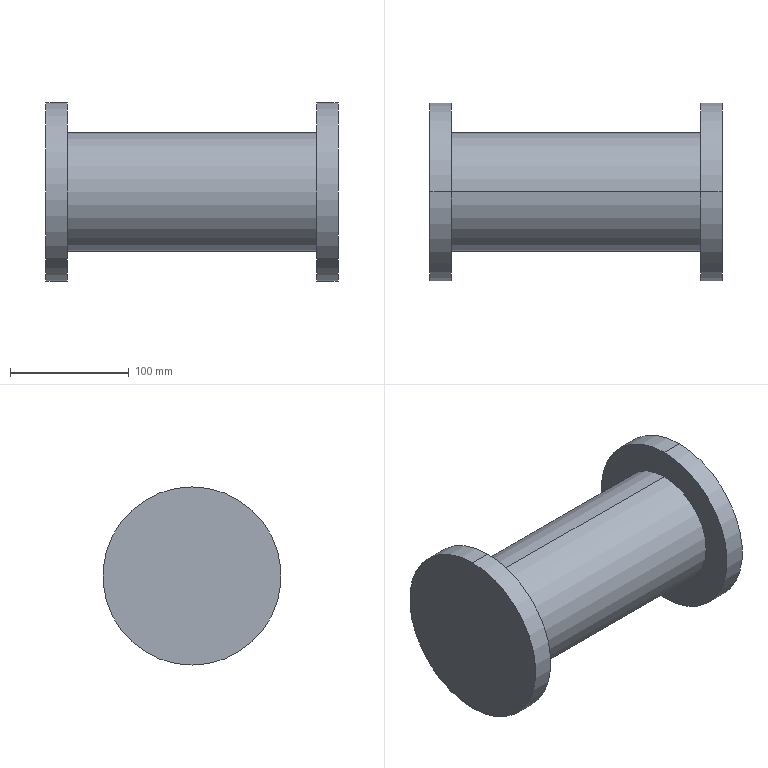Part | SolidWorks | features ICE 2, Extrusion 1 | 1 solid | 10 faces | box 246 x 150 x 150 mm | volume 2285509 mm3 | cylinder 6 | plane 4 | commonest cylinder face diameters 150 x4 100 x2
STEP:
#1=CARTESIAN_POINT('',(-228.,0.,-75.));
#2=VERTEX_POINT('',#1);
#3=CARTESIAN_POINT('',(-228.,0.,75.));
#4=VERTEX_POINT('',#3);
#5=CARTESIAN_POINT('',(-228.,0.,0.));
#6=DIRECTION('',(1.,0.,0.));
#7=DIRECTION('',(0.,0.,-1.));
#8=AXIS2_PLACEMENT_3D('',#5,#6,#7);
#9=CIRCLE('',#8,75.);
#10=EDGE_CURVE('',#2,#4,#9,.T.);
#11=ORIENTED_EDGE('',*,*,#10,.T.);
#12=CARTESIAN_POINT('',(-210.,0.,75.));
#13=VERTEX_POINT('',#12);
#14=CARTESIAN_POINT('',(-228.,0.,75.));
#15=DIRECTION('',(1.,0.,0.));
#16=VECTOR('',#15,1000.);
#17=LINE('',#14,#16);
#18=EDGE_CURVE('',#4,#13,#17,.T.);
#19=ORIENTED_EDGE('',*,*,#18,.T.);
#20=CARTESIAN_POINT('',(-210.,0.,-75.));
#21=VERTEX_POINT('',#20);
#22=CARTESIAN_POINT('',(-210.,0.,0.));
#23=DIRECTION('',(1.,0.,0.));
#24=DIRECTION('',(0.,0.,-1.));
#25=AXIS2_PLACEMENT_3D('',#22,#23,#24);
#26=CIRCLE('',#25,75.);
#27=EDGE_CURVE('',#21,#13,#26,.T.);
#28=ORIENTED_EDGE('',*,*,#27,.F.);
#29=CARTESIAN_POINT('',(-228.,0.,-75.));
#30=DIRECTION('',(1.,0.,0.));
#31=VECTOR('',#30,1000.);
#32=LINE('',#29,#31);
#33=EDGE_CURVE('',#2,#21,#32,.T.);
#34=ORIENTED_EDGE('',*,*,#33,.F.);
#35=EDGE_LOOP('',(#11,#19,#28,#34));
#36=FACE_OUTER_BOUND('',#35,.T.);
#37=CARTESIAN_POINT('',(-228.,0.,0.));
#38=DIRECTION('',(1.,0.,0.));
#39=DIRECTION('',(0.,0.,-1.));
#40=AXIS2_PLACEMENT_3D('',#37,#38,#39);
#41=CYLINDRICAL_SURFACE('',#40,75.);
#42=ADVANCED_FACE('',(#36),#41,.T.);
#43=CARTESIAN_POINT('',(-210.,0.,-50.));
#44=VERTEX_POINT('',#43);
#45=CARTESIAN_POINT('',(-210.,0.,50.));
#46=VERTEX_POINT('',#45);
#47=CARTESIAN_POINT('',(-210.,0.,0.));
#48=DIRECTION('',(1.,0.,0.));
#49=DIRECTION('',(0.,0.,-1.));
#50=AXIS2_PLACEMENT_3D('',#47,#48,#49);
#51=CIRCLE('',#50,50.);
#52=EDGE_CURVE('',#44,#46,#51,.T.);
#53=ORIENTED_EDGE('',*,*,#52,.T.);
#54=CARTESIAN_POINT('',(0.,0.,50.));
#55=VERTEX_POINT('',#54);
#56=CARTESIAN_POINT('',(-210.,0.,50.));
#57=DIRECTION('',(1.,0.,0.));
#58=VECTOR('',#57,1000.);
#59=LINE('',#56,#58);
#60=EDGE_CURVE('',#46,#55,#59,.T.);
#61=ORIENTED_EDGE('',*,*,#60,.T.);
#62=CARTESIAN_POINT('',(0.,0.,-50.));
#63=VERTEX_POINT('',#62);
#64=CARTESIAN_POINT('',(0.,0.,0.));
#65=DIRECTION('',(1.,0.,0.));
#66=DIRECTION('',(0.,0.,-1.));
#67=AXIS2_PLACEMENT_3D('',#64,#65,#66);
#68=CIRCLE('',#67,50.);
#69=EDGE_CURVE('',#63,#55,#68,.T.);
#70=ORIENTED_EDGE('',*,*,#69,.F.);
#71=CARTESIAN_POINT('',(-210.,0.,-50.));
#72=DIRECTION('',(1.,0.,0.));
#73=VECTOR('',#72,1000.);
#74=LINE('',#71,#73);
#75=EDGE_CURVE('',#44,#63,#74,.T.);
#76=ORIENTED_EDGE('',*,*,#75,.F.);
#77=EDGE_LOOP('',(#53,#61,#70,#76));
#78=FACE_OUTER_BOUND('',#77,.T.);
#79=CARTESIAN_POINT('',(-210.,0.,0.));
#80=DIRECTION('',(1.,0.,0.));
#81=DIRECTION('',(0.,0.,-1.));
#82=AXIS2_PLACEMENT_3D('',#79,#80,#81);
#83=CYLINDRICAL_SURFACE('',#82,50.);
#84=ADVANCED_FACE('',(#78),#83,.T.);
#85=CARTESIAN_POINT('',(18.,0.,-75.));
#86=VERTEX_POINT('',#85);
#87=CARTESIAN_POINT('',(18.,0.,75.));
#88=VERTEX_POINT('',#87);
#89=CARTESIAN_POINT('',(18.,0.,0.));
#90=DIRECTION('',(1.,0.,0.));
#91=DIRECTION('',(0.,0.,-1.));
#92=AXIS2_PLACEMENT_3D('',#89,#90,#91);
#93=CIRCLE('',#92,75.);
#94=EDGE_CURVE('',#86,#88,#93,.T.);
#95=ORIENTED_EDGE('',*,*,#94,.F.);
#96=CARTESIAN_POINT('',(0.,0.,-75.));
#97=VERTEX_POINT('',#96);
#98=CARTESIAN_POINT('',(18.,0.,-75.));
#99=DIRECTION('',(-1.,0.,0.));
#100=VECTOR('',#99,1000.);
#101=LINE('',#98,#100);
#102=EDGE_CURVE('',#86,#97,#101,.T.);
#103=ORIENTED_EDGE('',*,*,#102,.T.);
#104=CARTESIAN_POINT('',(0.,0.,75.));
#105=VERTEX_POINT('',#104);
#106=CARTESIAN_POINT('',(0.,0.,0.));
#107=DIRECTION('',(1.,0.,0.));
#108=DIRECTION('',(0.,0.,-1.));
#109=AXIS2_PLACEMENT_3D('',#106,#107,#108);
#110=CIRCLE('',#109,75.);
#111=EDGE_CURVE('',#97,#105,#110,.T.);
#112=ORIENTED_EDGE('',*,*,#111,.T.);
#113=CARTESIAN_POINT('',(18.,0.,75.));
#114=DIRECTION('',(-1.,0.,0.));
#115=VECTOR('',#114,1000.);
#116=LINE('',#113,#115);
#117=EDGE_CURVE('',#88,#105,#116,.T.);
#118=ORIENTED_EDGE('',*,*,#117,.F.);
#119=EDGE_LOOP('',(#95,#103,#112,#118));
#120=FACE_OUTER_BOUND('',#119,.T.);
#121=CARTESIAN_POINT('',(18.,0.,0.));
#122=DIRECTION('',(-1.,0.,0.));
#123=DIRECTION('',(0.,0.,1.));
#124=AXIS2_PLACEMENT_3D('',#121,#122,#123);
#125=CYLINDRICAL_SURFACE('',#124,75.);
#126=ADVANCED_FACE('',(#120),#125,.T.);
#127=ORIENTED_EDGE('',*,*,#102,.F.);
#128=CARTESIAN_POINT('',(18.,0.,0.));
#129=DIRECTION('',(1.,0.,0.));
#130=DIRECTION('',(0.,0.,-1.));
#131=AXIS2_PLACEMENT_3D('',#128,#129,#130);
#132=CIRCLE('',#131,75.);
#133=EDGE_CURVE('',#88,#86,#132,.T.);
#134=ORIENTED_EDGE('',*,*,#133,.F.);
#135=ORIENTED_EDGE('',*,*,#117,.T.);
#136=CARTESIAN_POINT('',(0.,0.,0.));
#137=DIRECTION('',(1.,0.,0.));
#138=DIRECTION('',(0.,0.,-1.));
#139=AXIS2_PLACEMENT_3D('',#136,#137,#138);
#140=CIRCLE('',#139,75.);
#141=EDGE_CURVE('',#105,#97,#140,.T.);
#142=ORIENTED_EDGE('',*,*,#141,.T.);
#143=EDGE_LOOP('',(#127,#134,#135,#142));
#144=FACE_OUTER_BOUND('',#143,.T.);
#145=CARTESIAN_POINT('',(18.,0.,0.));
#146=DIRECTION('',(-1.,0.,0.));
#147=DIRECTION('',(0.,0.,1.));
#148=AXIS2_PLACEMENT_3D('',#145,#146,#147);
#149=CYLINDRICAL_SURFACE('',#148,75.);
#150=ADVANCED_FACE('',(#144),#149,.T.);
#151=ORIENTED_EDGE('',*,*,#69,.T.);
#152=CARTESIAN_POINT('',(0.,0.,0.));
#153=DIRECTION('',(1.,0.,0.));
#154=DIRECTION('',(0.,0.,-1.));
#155=AXIS2_PLACEMENT_3D('',#152,#153,#154);
#156=CIRCLE('',#155,50.);
#157=EDGE_CURVE('',#55,#63,#156,.T.);
#158=ORIENTED_EDGE('',*,*,#157,.T.);
#159=EDGE_LOOP('',(#151,#158));
#160=FACE_BOUND('',#159,.T.);
#161=ORIENTED_EDGE('',*,*,#141,.F.);
#162=ORIENTED_EDGE('',*,*,#111,.F.);
#163=EDGE_LOOP('',(#161,#162));
#164=FACE_OUTER_BOUND('',#163,.T.);
#165=CARTESIAN_POINT('',(0.,0.,0.));
#166=DIRECTION('',(1.,0.,0.));
#167=DIRECTION('',(0.,0.,-1.));
#168=AXIS2_PLACEMENT_3D('',#165,#166,#167);
#169=PLANE('',#168);
#170=ADVANCED_FACE('',(#160,#164),#169,.F.);
#171=ORIENTED_EDGE('',*,*,#133,.T.);
#172=ORIENTED_EDGE('',*,*,#94,.T.);
#173=EDGE_LOOP('',(#171,#172));
#174=FACE_OUTER_BOUND('',#173,.T.);
#175=CARTESIAN_POINT('',(18.,0.,0.));
#176=DIRECTION('',(1.,0.,0.));
#177=DIRECTION('',(0.,0.,-1.));
#178=AXIS2_PLACEMENT_3D('',#175,#176,#177);
#179=PLANE('',#178);
#180=ADVANCED_FACE('',(#174),#179,.T.);
#181=ORIENTED_EDGE('',*,*,#60,.F.);
#182=CARTESIAN_POINT('',(-210.,0.,0.));
#183=DIRECTION('',(1.,0.,0.));
#184=DIRECTION('',(0.,0.,-1.));
#185=AXIS2_PLACEMENT_3D('',#182,#183,#184);
#186=CIRCLE('',#185,50.);
#187=EDGE_CURVE('',#46,#44,#186,.T.);
#188=ORIENTED_EDGE('',*,*,#187,.T.);
#189=ORIENTED_EDGE('',*,*,#75,.T.);
#190=ORIENTED_EDGE('',*,*,#157,.F.);
#191=EDGE_LOOP('',(#181,#188,#189,#190));
#192=FACE_OUTER_BOUND('',#191,.T.);
#193=CARTESIAN_POINT('',(-210.,0.,0.));
#194=DIRECTION('',(1.,0.,0.));
#195=DIRECTION('',(0.,0.,-1.));
#196=AXIS2_PLACEMENT_3D('',#193,#194,#195);
#197=CYLINDRICAL_SURFACE('',#196,50.);
#198=ADVANCED_FACE('',(#192),#197,.T.);
#199=ORIENTED_EDGE('',*,*,#18,.F.);
#200=CARTESIAN_POINT('',(-228.,0.,0.));
#201=DIRECTION('',(1.,0.,0.));
#202=DIRECTION('',(0.,0.,-1.));
#203=AXIS2_PLACEMENT_3D('',#200,#201,#202);
#204=CIRCLE('',#203,75.);
#205=EDGE_CURVE('',#4,#2,#204,.T.);
#206=ORIENTED_EDGE('',*,*,#205,.T.);
#207=ORIENTED_EDGE('',*,*,#33,.T.);
#208=CARTESIAN_POINT('',(-210.,0.,0.));
#209=DIRECTION('',(1.,0.,0.));
#210=DIRECTION('',(0.,0.,-1.));
#211=AXIS2_PLACEMENT_3D('',#208,#209,#210);
#212=CIRCLE('',#211,75.);
#213=EDGE_CURVE('',#13,#21,#212,.T.);
#214=ORIENTED_EDGE('',*,*,#213,.F.);
#215=EDGE_LOOP('',(#199,#206,#207,#214));
#216=FACE_OUTER_BOUND('',#215,.T.);
#217=CARTESIAN_POINT('',(-228.,0.,0.));
#218=DIRECTION('',(1.,0.,0.));
#219=DIRECTION('',(0.,0.,-1.));
#220=AXIS2_PLACEMENT_3D('',#217,#218,#219);
#221=CYLINDRICAL_SURFACE('',#220,75.);
#222=ADVANCED_FACE('',(#216),#221,.T.);
#223=ORIENTED_EDGE('',*,*,#10,.F.);
#224=ORIENTED_EDGE('',*,*,#205,.F.);
#225=EDGE_LOOP('',(#223,#224));
#226=FACE_OUTER_BOUND('',#225,.T.);
#227=CARTESIAN_POINT('',(-228.,0.,0.));
#228=DIRECTION('',(1.,0.,0.));
#229=DIRECTION('',(0.,0.,-1.));
#230=AXIS2_PLACEMENT_3D('',#227,#228,#229);
#231=PLANE('',#230);
#232=ADVANCED_FACE('',(#226),#231,.F.);
#233=ORIENTED_EDGE('',*,*,#52,.F.);
#234=ORIENTED_EDGE('',*,*,#187,.F.);
#235=EDGE_LOOP('',(#233,#234));
#236=FACE_BOUND('',#235,.T.);
#237=ORIENTED_EDGE('',*,*,#27,.T.);
#238=ORIENTED_EDGE('',*,*,#213,.T.);
#239=EDGE_LOOP('',(#237,#238));
#240=FACE_OUTER_BOUND('',#239,.T.);
#241=CARTESIAN_POINT('',(-210.,0.,0.));
#242=DIRECTION('',(1.,0.,0.));
#243=DIRECTION('',(0.,0.,-1.));
#244=AXIS2_PLACEMENT_3D('',#241,#242,#243);
#245=PLANE('',#244);
#246=ADVANCED_FACE('',(#236,#240),#245,.T.);
#247=CLOSED_SHELL('',(#42,#84,#126,#150,#170,#180,#198,#222,#232,#246));
#248=MANIFOLD_SOLID_BREP('',#247);
#249=CARTESIAN_POINT('',(0.,0.,0.));
#250=DIRECTION('',(0.,0.,1.));
#251=DIRECTION('',(1.,0.,0.));
#252=AXIS2_PLACEMENT_3D('',#249,#250,#251);
#253=(LENGTH_UNIT()NAMED_UNIT(*)SI_UNIT(.MILLI.,.METRE.));
#254=UNCERTAINTY_MEASURE_WITH_UNIT(LENGTH_MEASURE(0.00001),#253,'','');
#255=(NAMED_UNIT(*)PLANE_ANGLE_UNIT()SI_UNIT($,.RADIAN.));
#256=(NAMED_UNIT(*)SI_UNIT($,.STERADIAN.)SOLID_ANGLE_UNIT());
#257=(GEOMETRIC_REPRESENTATION_CONTEXT(3)GLOBAL_UNCERTAINTY_ASSIGNED_CONTEXT((#254))GLOBAL_UNIT_ASSIGNED_CONTEXT((#253,#255,#256))REPRESENTATION_CONTEXT('',''));
#258=ADVANCED_BREP_SHAPE_REPRESENTATION('',(#248,#252),#257);